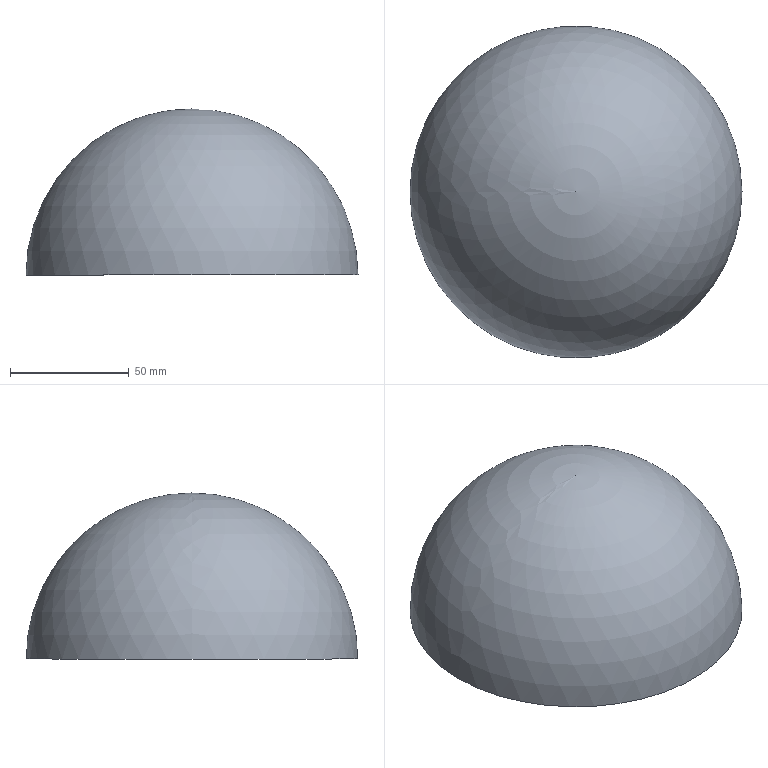Part | SolidWorks | features Revolution 1 | 1 solid | 2 faces | box 140 x 140 x 70 mm | volume 718378 mm3 | sphere 1 | plane 1
STEP:
#1=CARTESIAN_POINT('',(-70.,0.,0.));
#2=VERTEX_POINT('',#1);
#3=CARTESIAN_POINT('',(70.,0.,0.));
#4=VERTEX_POINT('',#3);
#5=CARTESIAN_POINT('',(0.,0.,0.));
#6=DIRECTION('',(0.,0.,-1.));
#7=DIRECTION('',(-1.,0.,0.));
#8=AXIS2_PLACEMENT_3D('',#5,#6,#7);
#9=CIRCLE('',#8,70.);
#10=EDGE_CURVE('',#2,#4,#9,.T.);
#11=ORIENTED_EDGE('',*,*,#10,.F.);
#12=CARTESIAN_POINT('',(0.,0.,0.));
#13=DIRECTION('',(0.,0.,-1.));
#14=DIRECTION('',(-1.,0.,0.));
#15=AXIS2_PLACEMENT_3D('',#12,#13,#14);
#16=CIRCLE('',#15,70.);
#17=EDGE_CURVE('',#4,#2,#16,.T.);
#18=ORIENTED_EDGE('',*,*,#17,.F.);
#19=EDGE_LOOP('',(#11,#18));
#20=FACE_OUTER_BOUND('',#19,.T.);
#21=CARTESIAN_POINT('',(0.,0.,0.));
#22=DIRECTION('',(0.,0.,1.));
#23=DIRECTION('',(-1.,0.,0.));
#24=AXIS2_PLACEMENT_3D('',#21,#22,#23);
#25=SPHERICAL_SURFACE('',#24,70.);
#26=ADVANCED_FACE('',(#20),#25,.T.);
#27=ORIENTED_EDGE('',*,*,#10,.T.);
#28=ORIENTED_EDGE('',*,*,#17,.T.);
#29=EDGE_LOOP('',(#27,#28));
#30=FACE_OUTER_BOUND('',#29,.T.);
#31=CARTESIAN_POINT('',(0.,0.,0.));
#32=DIRECTION('',(0.,0.,-1.));
#33=DIRECTION('',(-1.,0.,0.));
#34=AXIS2_PLACEMENT_3D('',#31,#32,#33);
#35=PLANE('',#34);
#36=ADVANCED_FACE('',(#30),#35,.T.);
#37=CLOSED_SHELL('',(#26,#36));
#38=MANIFOLD_SOLID_BREP('',#37);
#39=CARTESIAN_POINT('',(0.,0.,0.));
#40=DIRECTION('',(0.,0.,1.));
#41=DIRECTION('',(1.,0.,0.));
#42=AXIS2_PLACEMENT_3D('',#39,#40,#41);
#43=(LENGTH_UNIT()NAMED_UNIT(*)SI_UNIT(.MILLI.,.METRE.));
#44=UNCERTAINTY_MEASURE_WITH_UNIT(LENGTH_MEASURE(0.00001),#43,'','');
#45=(NAMED_UNIT(*)PLANE_ANGLE_UNIT()SI_UNIT($,.RADIAN.));
#46=(NAMED_UNIT(*)SI_UNIT($,.STERADIAN.)SOLID_ANGLE_UNIT());
#47=(GEOMETRIC_REPRESENTATION_CONTEXT(3)GLOBAL_UNCERTAINTY_ASSIGNED_CONTEXT((#44))GLOBAL_UNIT_ASSIGNED_CONTEXT((#43,#45,#46))REPRESENTATION_CONTEXT('',''));
#48=ADVANCED_BREP_SHAPE_REPRESENTATION('',(#38,#42),#47);